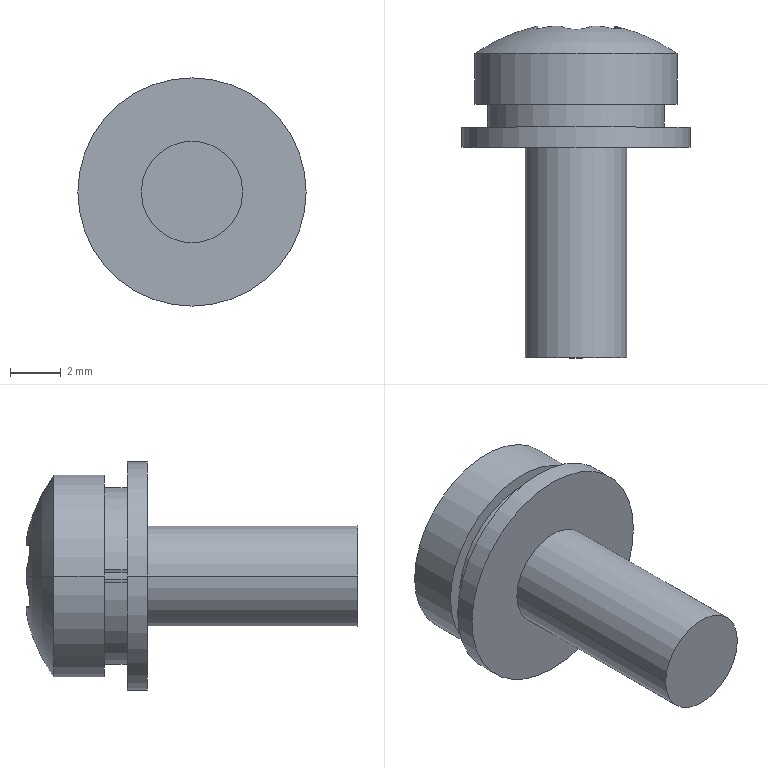Part | STEP file | LIB_28112301_M4X10 | 1 solid | 29 faces | box 9 x 13.088 x 9 mm | volume 307.834 mm3 | cylinder 20 | plane 7 | sphere 2 | commonest cylinder face diameters 0.992 x6 1.2 x6 4 x3 8 x2 9 x2 7 x1